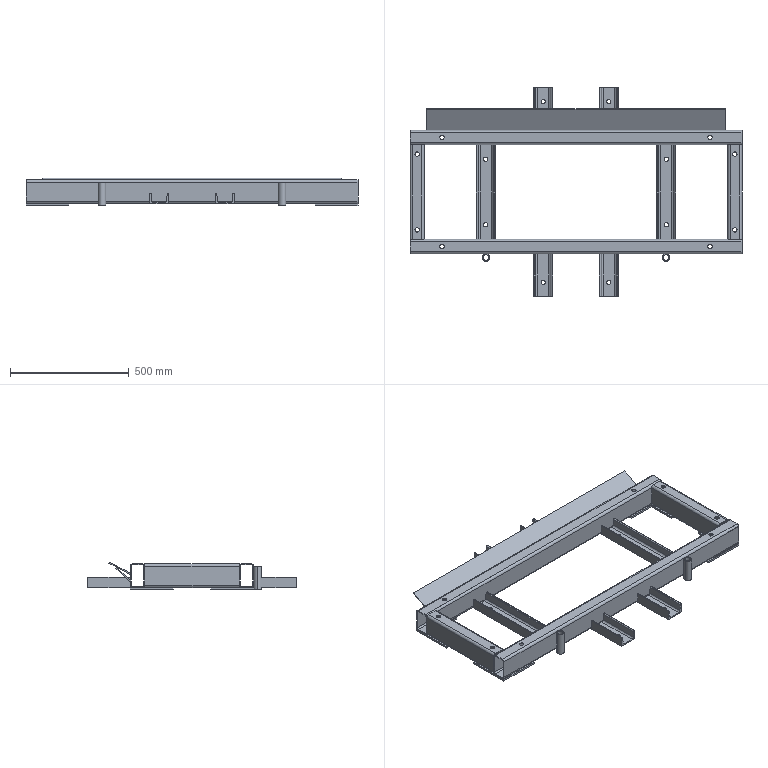Part | SolidWorks | features ICE 4, HoleWzd 2, WeldMemberFeat 2, LPattern 1, MoveCopyBody 1, WeldmentFeature 1 | 20 solids | 288 faces | box 1400 x 880 x 118 mm | volume 7030026 mm3 | plane 160 | cylinder 128 | commonest cylinder face diameters 18 x64 12 x16 20 x16 8 x12 16 x12 24 x4